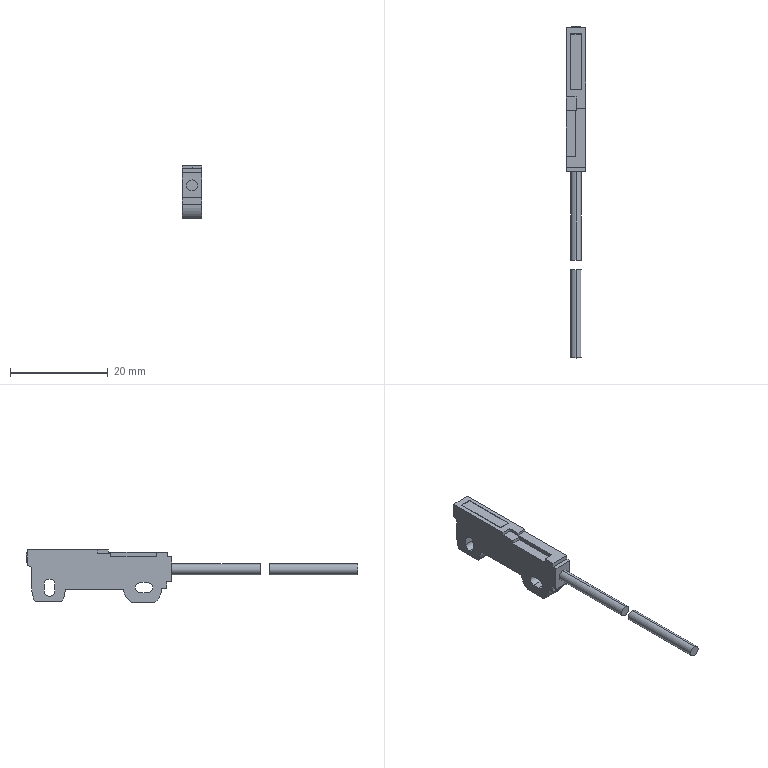Part | SolidWorks | features BaseBody 2 | 2 solids | 73 faces | box 4 x 67.8 x 10.654 mm | volume 1071 mm3 | plane 55 | cylinder 18 | commonest cylinder face diameters 2.1 x5 3.6 x5 2.2 x4 6.245 x1 7.045 x1 7.2 x1